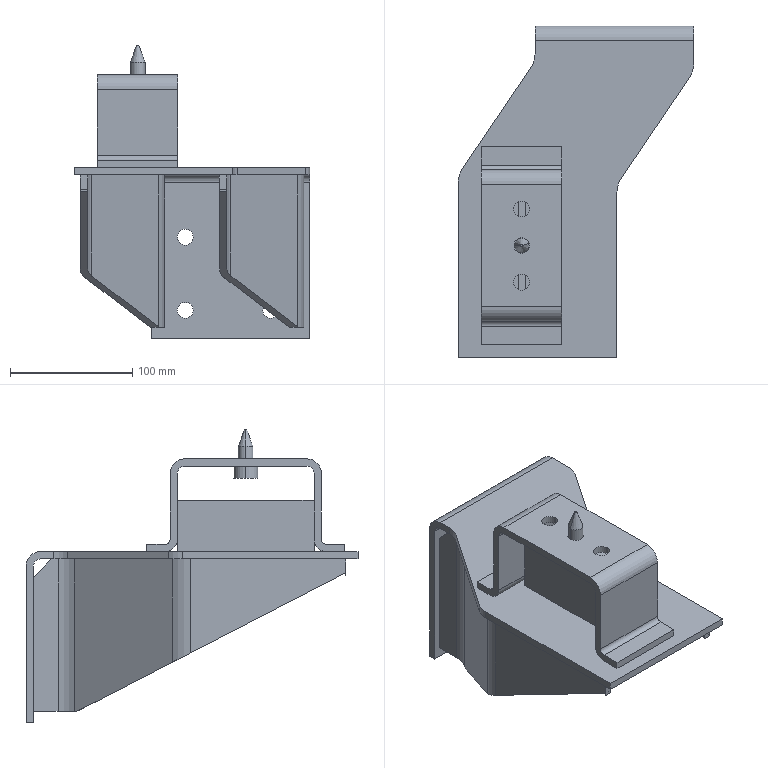Part | NX | features BREP 6 | 6 solids | 104 faces | box 193 x 272 x 240 mm | volume 714638 mm3 | plane 61 | cylinder 40 | cone 3 | commonest cylinder face diameters 13 x12 40 x6 12 x5 20 x4 24 x3 8 x2